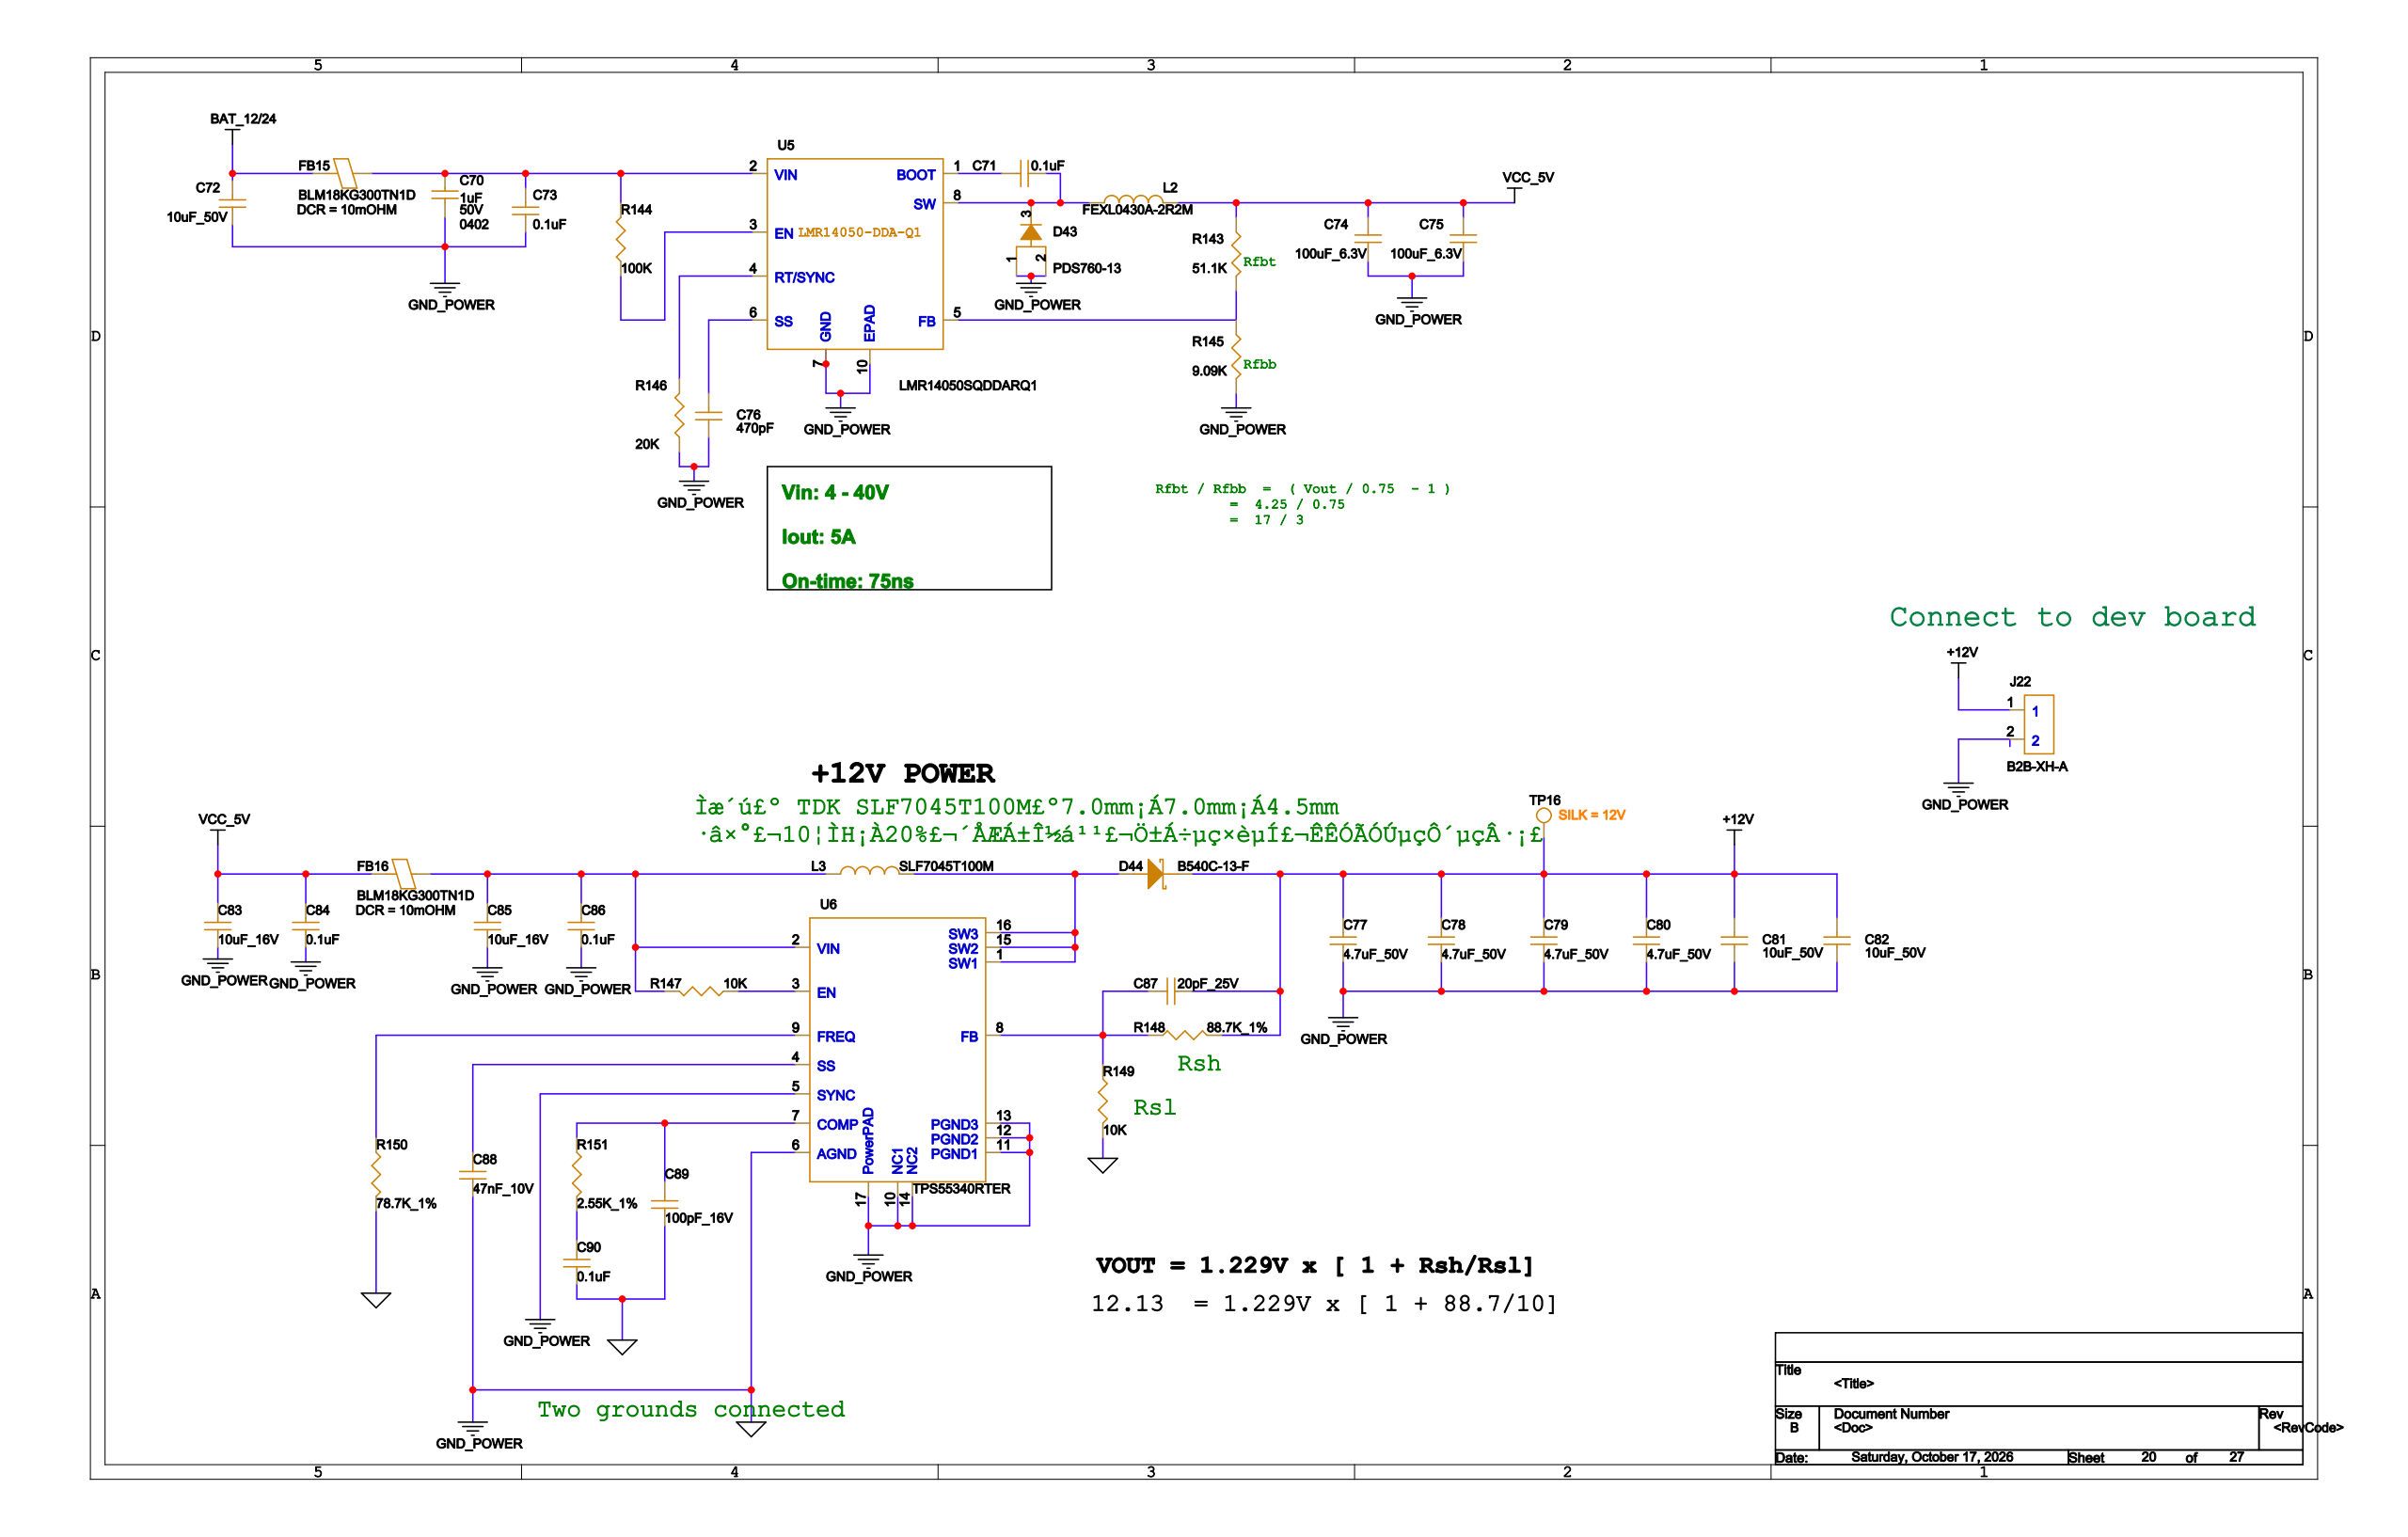Circuit board | Cadence Allegro | 477 parts | 327 nets | one sheet of the schematic
Parts on this sheet (reference | value | footprint):
C70 | 1uF | 0402
C71 | 0.1uF | 0402
C72 | 10uF_50V | 1206
C73 | 0.1uF | 0402
C74 | 100uF_6.3V | 1206
C75 | 100uF_6.3V | 1206
C76 | 470pF | 0402
C77 | 4.7uF_50V | 1210
C78 | 4.7uF_50V | 1210
C79 | 4.7uF_50V | 1210
C80 | 4.7uF_50V | 1210
C81 | 10uF_50V | 1206
C82 | 10uF_50V | 1206
C83 | 10uF_16V | 0603
C84 | 0.1uF | 0402
C85 | 10uF_16V | 0603
C86 | 0.1uF | 0402
C87 | 20pF_25V | 0402
C88 | 47nF_10V | 0402
C89 | 100pF_16V | 0402
C90 | 0.1uF | 0402
D43 | PDS760-13 | PDS760
D44 | B540C-13-F | SMC
FB15 | BLM18KG300TN1D | 0603
FB16 | BLM18KG300TN1D | 0603
J22 | B2B-XH-A | B2B-XH-A
L2 | FEXL0430A-2R2M | L_41X41_H210_BOURNS
L3 | SLF7045T100M | SMD_7X7
R143 | 51.1K | 0402
R144 | 100K | 0402
R145 | 9.09K | 0402
R146 | 20K | 0402
R147 | 10K | 0402
R148 | 88.7K_1% | 0402
R149 | 10K | 0402
R150 | 78.7K_1% | 0402
R151 | 2.55K_1% | 0402
TP16 | TP | S0400CI
U5 | LMR14050SQDDARQ1 | SOP8P_60_PAD29X21_127_H170
U6 | TPS55340RTER | WQFN16-3X3
Nets of these parts (net: part-pin ...):
BAT_GND: C70-2 C72-1 C73-1 C74-2 C75-2 C76-1 C77-1 C78-1 C79-1 C80-1 C81-1 C82-1 C83-1 C84-1 C85-1 C86-1 C88-1 C89-1 C90-1 D43-1 D43-2 J22-2 R145-2 R146-1 R149-2 R150-2 U5-7 U5-10 U6-5 U6-6 U6-10 U6-11 U6-12 U6-13 U6-14 U6-17
BAT_12/24: C72-2 FB15-2
+12V: C77-2 C78-2 C79-2 C80-2 C81-2 C82-2 C87-1 D44-1 J22-1 R148-2 TP16-1
N16895476: C87-2 R148-1 R149-1 U6-8
N16895519: C88-2 U6-4
N16895535: C89-2 R151-1 U6-7
N16894931: C70-1 C73-2 FB15-1 R144-2 U5-2
N16895273: D44-2 L3-2 U6-1 U6-15 U6-16
N16895259: C85-2 C86-2 FB16-1 L3-1 R147-2 U6-2
N16895056: R144-1 U5-3
N16895096: R146-2 U5-4
N16895474: R147-1 U6-3
N16895507: R150-1 U6-9
N16895605: C90-2 R151-2
N16894945: C71-1 D43-3 L2-1 U5-8
VCC_5V: C74-1 C75-1 C83-2 C84-2 FB16-2 L2-2 R143-1
N16895125: C76-2 U5-6
N16895118: R143-2 R145-1 U5-5
N16894943: C71-2 U5-1